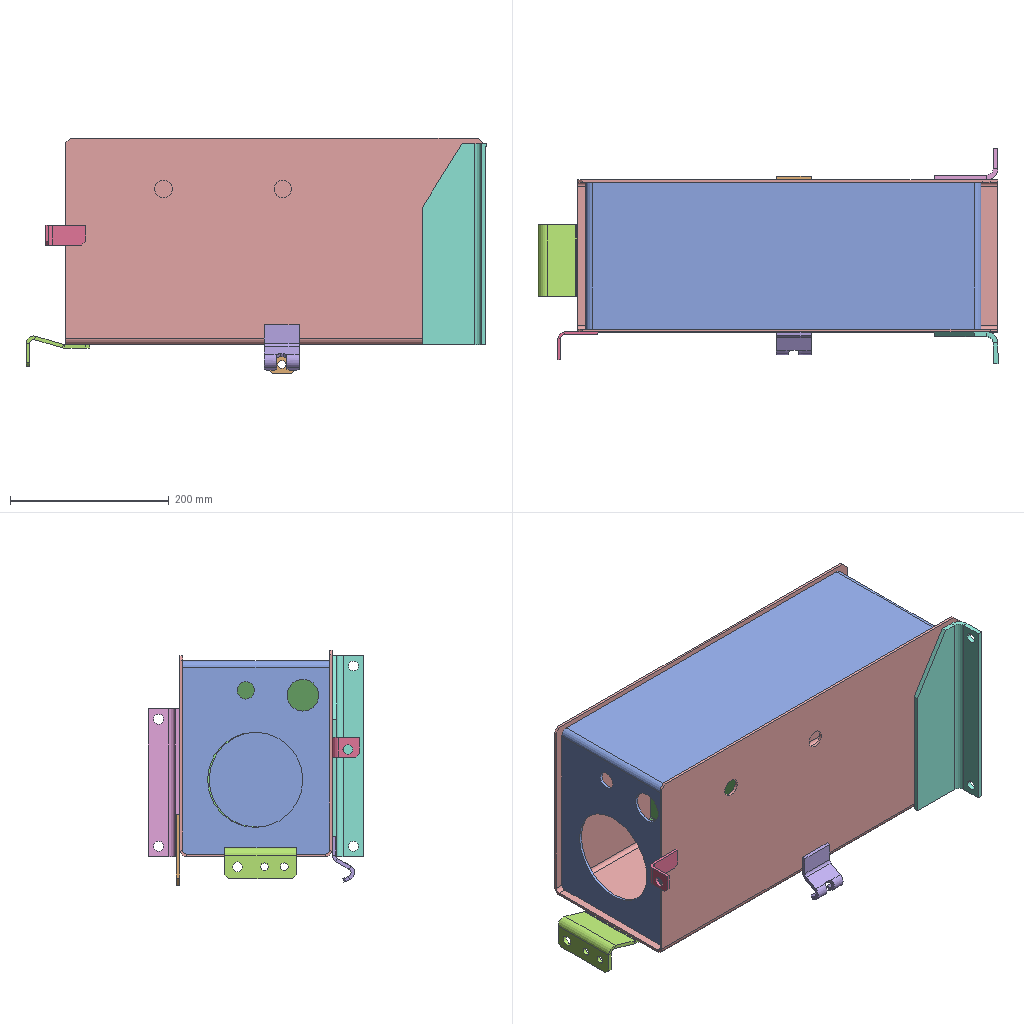Assembly | SolidWorks | 9 different items | 9 placed | box 579 x 271 x 297 mm
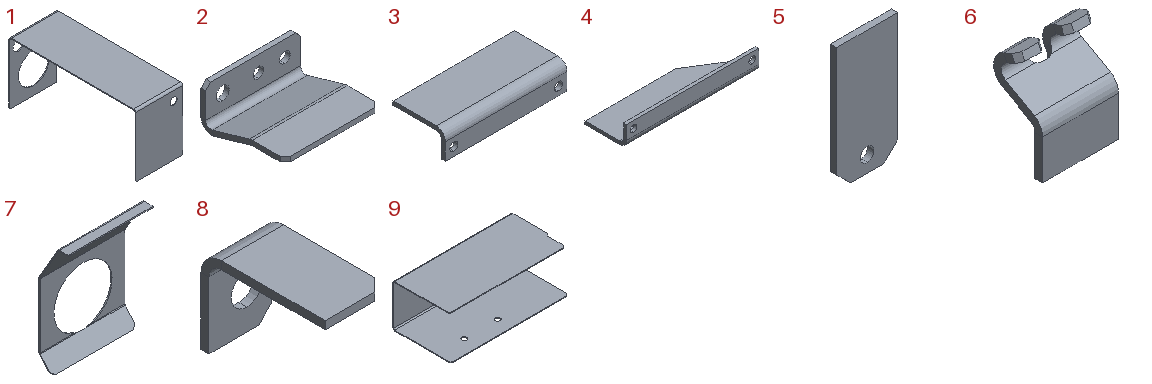Parts list (item | quantity | size | volume | features):
1 | x1 | 185 x 497.4 x 243.2 mm | 531785 mm3 | features ICE 2, Fillet 1, FlatPattern 1, SMBaseFlange 1, SheetMetal 1
2 | x1 | 90 x 80 x 38.833 mm | 44176 mm3 | features Chamfer 1, FlatPattern 1, ICE 1, SMBaseFlange 1, SheetMetal 1
3 | x1 | 186 x 80 x 40 mm | 120482 mm3 | features FlatPattern 1, ICE 1, SMBaseFlange 1, SheetMetal 1
4 | x1 | 253 x 80 x 40 mm | 152413 mm3 | features ICE 2, FlatPattern 1, SMBaseFlange 1, SheetMetal 1
5 | x1 | 44 x 4.5 x 90 mm | 17017 mm3 | features FlatPattern 1, SMBaseFlange 1, SheetMetal 1
6 | x1 | 44 x 28.417 x 57.001 mm | 13183 mm3 | features Chamfer 1, Fillet 1, FlatPattern 1, ICE 1, SMBaseFlange 1, SheetMetal 1
7 | x1 | 175 x 60.3 x 234.795 mm | 83264 mm3 | features Chamfer 1, FlatPattern 1, Fold 1, ICE 1, SMBaseFlange 1, SheetMetal 1, UnFold 1
8 | x1 | 25 x 50 x 35 mm | 5845 mm3 | features Chamfer 1, FlatPattern 1, ICE 1, SMBaseFlange 1, SheetMetal 1
9 | x1 | 529 x 260 x 191.4 mm | 1146717 mm3 | features Chamfer 3, ICE 3, FlatPattern 1, SMBaseFlange 1, SheetMetal 1
Mates (type | each side: item.copy, entity, surface, feature):
Coincident | 9.1 face plane Base-Flange1 | 1.1 face plane Base-Flange1 | 2 times
DistanceDim | 1.1 face plane Base-Flange1 | 9.1 face plane Base-Flange1
Coincident | 9.1 face plane Base-Flange1 | 2.1 face plane Base-Flange1
DistanceDim | 2.1 face plane Base-Flange1 | 9.1 face plane Base-Flange1
DistanceDim | 9.1 face plane Base-Flange1 | 2.1 face plane Base-Flange1
Coincident | 9.1 face plane Base-Flange1 | 3.1 face plane Base-Flange1 | 3 times
Coincident | 9.1 face plane Base-Flange1 | 4.1 face plane Base-Flange1 | 3 times
Coincident | 9.1 face plane Base-Flange1 | 5.1 face plane Base-Flange1
DistanceDim | 9.1 face plane Base-Flange1 | 5.1 face plane Base-Flange1
DistanceDim | 5.1 face cylinder Base-Flange1 | 9.1 face plane Base-Flange1
Coincident | 9.1 face plane Base-Flange1 | 6.1 face plane Base-Flange1
Coincident | 5.1 face plane Base-Flange1 | 6.1 face plane Base-Flange1
DistanceDim | 9.1 face plane Base-Flange1 | 6.1 face plane Base-Flange1
Coincident | 1.1 face plane Base-Flange1 | 7.1 face plane Base-Flange1
DistanceDim | 1.1 face plane Base-Flange1 | 7.1 face plane Base-Flange1 | 2 times
Coincident | 9.1 face plane Base-Flange1 | 8.1 face plane Base-Flange1
DistanceDim | 8.1 face plane Base-Flange1 | 9.1 face plane Base-Flange1
DistanceDim | 9.1 face plane Base-Flange1 | 8.1 face plane Base-Flange1